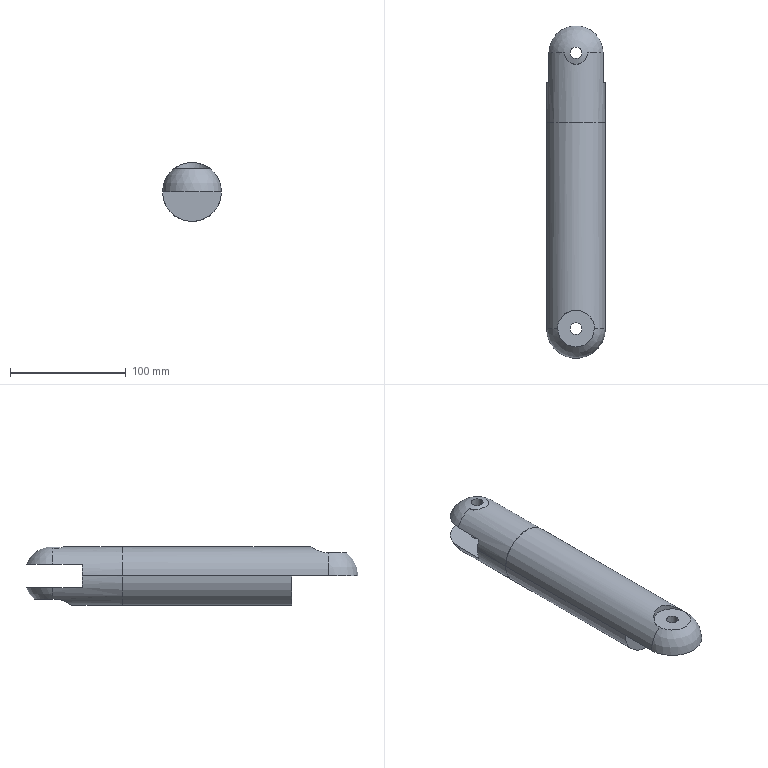Part | SolidWorks | features ICE 10, Fillet 1, MoveCopyBody 1, Revolution 1, Scale 1, Split 1 | 1 solid | 34 faces | box 50.8 x 286.949 x 50.8 mm | volume 448364 mm3 | cylinder 17 | plane 9 | sphere 3 | spline 3 | torus 2 | commonest cylinder face diameters 10.1 x6 50.8 x4 0.8 x2 32 x2 50 x2 20 x1